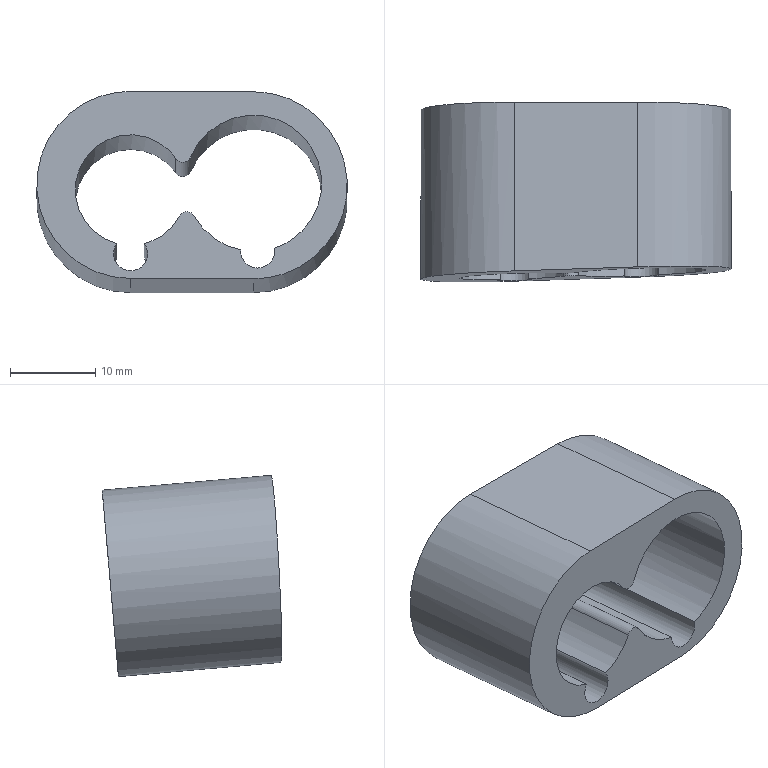Part | NX | features solid 2 | 1 solid | 14 faces | box 36.5 x 21.114 x 23.653 mm | volume 6698 mm3 | cylinder 10 | plane 4 | commonest cylinder face diameters 2 x2 4 x2 13 x2 16 x2 22 x2
STEP:
#1=CARTESIAN_POINT('',(-235.351,-38.939,-37.55));
#2=VERTEX_POINT('',#1);
#3=CARTESIAN_POINT('',(-229.897,-39.284,-41.487));
#4=VERTEX_POINT('',#3);
#5=CARTESIAN_POINT('',(-228.366,-38.599,-33.665));
#6=DIRECTION('',(0.,-0.9962,0.08716));
#7=DIRECTION('',(0.,-0.08716,-0.9962));
#8=AXIS2_PLACEMENT_3D('',#5,#6,#7);
#9=CIRCLE('',#8,8.);
#10=EDGE_CURVE('',#2,#4,#9,.T.);
#11=ORIENTED_EDGE('',*,*,#10,.F.);
#12=CARTESIAN_POINT('',(-235.351,-58.041,-35.879));
#13=VERTEX_POINT('',#12);
#14=CARTESIAN_POINT('',(-235.351,-58.346,-35.852));
#15=DIRECTION('',(0.,0.9962,-0.08716));
#16=VECTOR('',#15,1000.);
#17=LINE('',#14,#16);
#18=EDGE_CURVE('',#2,#13,#17,.F.);
#19=ORIENTED_EDGE('',*,*,#18,.T.);
#20=CARTESIAN_POINT('',(-229.897,-58.074,-39.843));
#21=VERTEX_POINT('',#20);
#22=CARTESIAN_POINT('',(-228.366,-57.608,-32.002));
#23=DIRECTION('',(-0.03252,0.9981,-0.05307));
#24=DIRECTION('',(0.6892,-0.01607,-0.7244));
#25=AXIS2_PLACEMENT_3D('',#22,#23,#24);
#26=ELLIPSE('',#25,8.009,8.);
#27=EDGE_CURVE('',#13,#21,#26,.F.);
#28=ORIENTED_EDGE('',*,*,#27,.T.);
#29=CARTESIAN_POINT('',(-229.897,-48.729,-40.661));
#30=DIRECTION('',(0.,0.9962,-0.08716));
#31=VECTOR('',#30,1000.);
#32=LINE('',#29,#31);
#33=EDGE_CURVE('',#21,#4,#32,.T.);
#34=ORIENTED_EDGE('',*,*,#33,.T.);
#35=EDGE_LOOP('',(#11,#19,#28,#34));
#36=FACE_BOUND('',#35,.T.);
#37=CARTESIAN_POINT('',(-228.366,-58.006,-31.967));
#38=DIRECTION('',(0.,0.9962,-0.08716));
#39=DIRECTION('',(-0.9997,-0.001977,-0.0226));
#40=AXIS2_PLACEMENT_3D('',#37,#38,#39);
#41=CYLINDRICAL_SURFACE('',#40,8.);
#42=ADVANCED_FACE('',(#36),#41,.F.);
#43=CARTESIAN_POINT('',(-237.502,-38.349,-30.804));
#44=VERTEX_POINT('',#43);
#45=CARTESIAN_POINT('',(-244.435,-39.222,-40.782));
#46=VERTEX_POINT('',#45);
#47=CARTESIAN_POINT('',(-242.835,-38.673,-34.506));
#48=DIRECTION('',(0.,-0.9962,0.08716));
#49=DIRECTION('',(0.,-0.08716,-0.9962));
#50=AXIS2_PLACEMENT_3D('',#47,#48,#49);
#51=CIRCLE('',#50,6.5);
#52=EDGE_CURVE('',#44,#46,#51,.T.);
#53=ORIENTED_EDGE('',*,*,#52,.F.);
#54=CARTESIAN_POINT('',(-237.502,-57.751,-29.107));
#55=VERTEX_POINT('',#54);
#56=CARTESIAN_POINT('',(-237.502,-58.196,-29.068));
#57=DIRECTION('',(0.,0.9962,-0.08716));
#58=VECTOR('',#57,1000.);
#59=LINE('',#56,#58);
#60=EDGE_CURVE('',#44,#55,#59,.F.);
#61=ORIENTED_EDGE('',*,*,#60,.T.);
#62=CARTESIAN_POINT('',(-244.435,-58.508,-39.095));
#63=VERTEX_POINT('',#62);
#64=CARTESIAN_POINT('',(-242.835,-58.122,-32.805));
#65=DIRECTION('',(-0.03252,0.9981,-0.05307));
#66=DIRECTION('',(0.6892,-0.01607,-0.7244));
#67=AXIS2_PLACEMENT_3D('',#64,#65,#66);
#68=ELLIPSE('',#67,6.507,6.5);
#69=EDGE_CURVE('',#55,#63,#68,.F.);
#70=ORIENTED_EDGE('',*,*,#69,.T.);
#71=CARTESIAN_POINT('',(-244.435,-49.107,-39.917));
#72=DIRECTION('',(0.,0.9962,-0.08716));
#73=VECTOR('',#72,1000.);
#74=LINE('',#71,#73);
#75=EDGE_CURVE('',#63,#46,#74,.T.);
#76=ORIENTED_EDGE('',*,*,#75,.T.);
#77=EDGE_LOOP('',(#53,#61,#70,#76));
#78=FACE_BOUND('',#77,.T.);
#79=CARTESIAN_POINT('',(-242.835,-58.52,-32.77));
#80=DIRECTION('',(0.,0.9962,-0.08716));
#81=DIRECTION('',(1.,0.,0.));
#82=AXIS2_PLACEMENT_3D('',#79,#80,#81);
#83=CYLINDRICAL_SURFACE('',#82,6.5);
#84=ADVANCED_FACE('',(#78),#83,.F.);
#85=CARTESIAN_POINT('',(-228.366,-39.579,-44.865));
#86=VERTEX_POINT('',#85);
#87=CARTESIAN_POINT('',(-228.366,-37.662,-22.949));
#88=VERTEX_POINT('',#87);
#89=CARTESIAN_POINT('',(-228.366,-38.62,-33.907));
#90=DIRECTION('',(0.,-0.9962,0.08716));
#91=DIRECTION('',(1.,0.,0.));
#92=AXIS2_PLACEMENT_3D('',#89,#90,#91);
#93=CIRCLE('',#92,11.);
#94=EDGE_CURVE('',#86,#88,#93,.T.);
#95=ORIENTED_EDGE('',*,*,#94,.T.);
#96=CARTESIAN_POINT('',(-228.366,-57.036,-21.254));
#97=VERTEX_POINT('',#96);
#98=CARTESIAN_POINT('',(-228.366,-57.586,-21.206));
#99=DIRECTION('',(0.,0.9962,-0.08716));
#100=VECTOR('',#99,1000.);
#101=LINE('',#98,#100);
#102=EDGE_CURVE('',#97,#88,#101,.T.);
#103=ORIENTED_EDGE('',*,*,#102,.F.);
#104=CARTESIAN_POINT('',(-228.366,-58.205,-43.235));
#105=VERTEX_POINT('',#104);
#106=CARTESIAN_POINT('',(-228.366,-57.621,-32.244));
#107=DIRECTION('',(-0.03252,0.9981,-0.05307));
#108=DIRECTION('',(0.6892,-0.01607,-0.7244));
#109=AXIS2_PLACEMENT_3D('',#106,#107,#108);
#110=ELLIPSE('',#109,11.012,11.);
#111=EDGE_CURVE('',#105,#97,#110,.F.);
#112=ORIENTED_EDGE('',*,*,#111,.F.);
#113=CARTESIAN_POINT('',(-228.366,-59.503,-43.122));
#114=DIRECTION('',(0.,0.9962,-0.08716));
#115=VECTOR('',#114,1000.);
#116=LINE('',#113,#115);
#117=EDGE_CURVE('',#105,#86,#116,.T.);
#118=ORIENTED_EDGE('',*,*,#117,.T.);
#119=EDGE_LOOP('',(#95,#103,#112,#118));
#120=FACE_BOUND('',#119,.T.);
#121=CARTESIAN_POINT('',(-228.366,-58.544,-32.164));
#122=DIRECTION('',(0.,0.9962,-0.08716));
#123=DIRECTION('',(0.,0.08716,0.9962));
#124=AXIS2_PLACEMENT_3D('',#121,#122,#123);
#125=CYLINDRICAL_SURFACE('',#124,11.);
#126=ADVANCED_FACE('',(#120),#125,.T.);
#127=CARTESIAN_POINT('',(-242.866,-37.662,-22.949));
#128=VERTEX_POINT('',#127);
#129=CARTESIAN_POINT('',(-242.866,-37.662,-22.949));
#130=DIRECTION('',(1.,0.,0.));
#131=VECTOR('',#130,1000.);
#132=LINE('',#129,#131);
#133=EDGE_CURVE('',#128,#88,#132,.T.);
#134=ORIENTED_EDGE('',*,*,#133,.F.);
#135=CARTESIAN_POINT('',(-242.866,-57.506,-21.212));
#136=VERTEX_POINT('',#135);
#137=CARTESIAN_POINT('',(-242.866,-57.586,-21.206));
#138=DIRECTION('',(0.,0.9962,-0.08716));
#139=VECTOR('',#138,1000.);
#140=LINE('',#137,#139);
#141=EDGE_CURVE('',#136,#128,#140,.T.);
#142=ORIENTED_EDGE('',*,*,#141,.F.);
#143=CARTESIAN_POINT('',(-242.869,-57.506,-21.212));
#144=DIRECTION('',(-0.9995,-0.03241,0.002836));
#145=VECTOR('',#144,1000.);
#146=LINE('',#143,#145);
#147=EDGE_CURVE('',#136,#97,#146,.F.);
#148=ORIENTED_EDGE('',*,*,#147,.T.);
#149=ORIENTED_EDGE('',*,*,#102,.T.);
#150=EDGE_LOOP('',(#134,#142,#148,#149));
#151=FACE_BOUND('',#150,.T.);
#152=CARTESIAN_POINT('',(-242.866,-57.586,-21.206));
#153=DIRECTION('',(0.,0.08716,0.9962));
#154=DIRECTION('',(1.,0.,0.));
#155=AXIS2_PLACEMENT_3D('',#152,#153,#154);
#156=PLANE('',#155);
#157=ADVANCED_FACE('',(#151),#156,.T.);
#158=CARTESIAN_POINT('',(-242.866,-39.579,-44.865));
#159=VERTEX_POINT('',#158);
#160=CARTESIAN_POINT('',(-242.866,-38.62,-33.907));
#161=DIRECTION('',(0.,-0.9962,0.08716));
#162=DIRECTION('',(1.,0.,0.));
#163=AXIS2_PLACEMENT_3D('',#160,#161,#162);
#164=CIRCLE('',#163,11.);
#165=EDGE_CURVE('',#128,#159,#164,.T.);
#166=ORIENTED_EDGE('',*,*,#165,.T.);
#167=CARTESIAN_POINT('',(-242.866,-58.675,-43.194));
#168=VERTEX_POINT('',#167);
#169=CARTESIAN_POINT('',(-242.866,-59.503,-43.122));
#170=DIRECTION('',(0.,0.9962,-0.08716));
#171=VECTOR('',#170,1000.);
#172=LINE('',#169,#171);
#173=EDGE_CURVE('',#168,#159,#172,.T.);
#174=ORIENTED_EDGE('',*,*,#173,.F.);
#175=CARTESIAN_POINT('',(-242.866,-58.091,-32.203));
#176=DIRECTION('',(-0.03252,0.9981,-0.05307));
#177=DIRECTION('',(0.6892,-0.01607,-0.7244));
#178=AXIS2_PLACEMENT_3D('',#175,#176,#177);
#179=ELLIPSE('',#178,11.012,11.);
#180=EDGE_CURVE('',#136,#168,#179,.F.);
#181=ORIENTED_EDGE('',*,*,#180,.F.);
#182=ORIENTED_EDGE('',*,*,#141,.T.);
#183=EDGE_LOOP('',(#166,#174,#181,#182));
#184=FACE_BOUND('',#183,.T.);
#185=CARTESIAN_POINT('',(-242.866,-58.544,-32.164));
#186=DIRECTION('',(0.,0.9962,-0.08716));
#187=DIRECTION('',(0.,0.08716,0.9962));
#188=AXIS2_PLACEMENT_3D('',#185,#186,#187);
#189=CYLINDRICAL_SURFACE('',#188,11.);
#190=ADVANCED_FACE('',(#184),#189,.T.);
#191=CARTESIAN_POINT('',(-228.366,-39.579,-44.865));
#192=DIRECTION('',(-1.,0.,0.));
#193=VECTOR('',#192,1000.);
#194=LINE('',#191,#193);
#195=EDGE_CURVE('',#86,#159,#194,.T.);
#196=ORIENTED_EDGE('',*,*,#195,.F.);
#197=ORIENTED_EDGE('',*,*,#117,.F.);
#198=CARTESIAN_POINT('',(-228.409,-58.206,-43.235));
#199=DIRECTION('',(0.9995,0.03241,-0.002836));
#200=VECTOR('',#199,1000.);
#201=LINE('',#198,#200);
#202=EDGE_CURVE('',#105,#168,#201,.F.);
#203=ORIENTED_EDGE('',*,*,#202,.T.);
#204=ORIENTED_EDGE('',*,*,#173,.T.);
#205=EDGE_LOOP('',(#196,#197,#203,#204));
#206=FACE_BOUND('',#205,.T.);
#207=CARTESIAN_POINT('',(-228.366,-59.503,-43.122));
#208=DIRECTION('',(0.,-0.08716,-0.9962));
#209=DIRECTION('',(-1.,0.,0.));
#210=AXIS2_PLACEMENT_3D('',#207,#208,#209);
#211=PLANE('',#210);
#212=ADVANCED_FACE('',(#206),#211,.T.);
#213=ORIENTED_EDGE('',*,*,#27,.F.);
#214=CARTESIAN_POINT('',(-237.106,-58.099,-35.889));
#215=VERTEX_POINT('',#214);
#216=CARTESIAN_POINT('',(-236.225,-58.096,-36.363));
#217=DIRECTION('',(-0.03252,0.9981,-0.05307));
#218=DIRECTION('',(0.6892,-0.01607,-0.7244));
#219=AXIS2_PLACEMENT_3D('',#216,#217,#218);
#220=ELLIPSE('',#219,1.001,1.);
#221=EDGE_CURVE('',#13,#215,#220,.F.);
#222=ORIENTED_EDGE('',*,*,#221,.T.);
#223=CARTESIAN_POINT('',(-241.235,-58.405,-39.104));
#224=VERTEX_POINT('',#223);
#225=CARTESIAN_POINT('',(-242.835,-58.122,-32.805));
#226=DIRECTION('',(-0.03252,0.9981,-0.05307));
#227=DIRECTION('',(0.6892,-0.01607,-0.7244));
#228=AXIS2_PLACEMENT_3D('',#225,#226,#227);
#229=ELLIPSE('',#228,6.507,6.5);
#230=EDGE_CURVE('',#224,#215,#229,.F.);
#231=ORIENTED_EDGE('',*,*,#230,.F.);
#232=CARTESIAN_POINT('',(-242.835,-58.52,-40.299));
#233=DIRECTION('',(-0.03252,0.9981,-0.05307));
#234=DIRECTION('',(0.6892,-0.01607,-0.7244));
#235=AXIS2_PLACEMENT_3D('',#232,#233,#234);
#236=ELLIPSE('',#235,2.002,2.);
#237=EDGE_CURVE('',#63,#224,#236,.F.);
#238=ORIENTED_EDGE('',*,*,#237,.F.);
#239=ORIENTED_EDGE('',*,*,#69,.F.);
#240=CARTESIAN_POINT('',(-235.758,-57.685,-28.923));
#241=VERTEX_POINT('',#240);
#242=CARTESIAN_POINT('',(-236.682,-57.694,-28.538));
#243=DIRECTION('',(-0.03252,0.9981,-0.05307));
#244=DIRECTION('',(-0.6892,0.01607,0.7244));
#245=AXIS2_PLACEMENT_3D('',#242,#243,#244);
#246=ELLIPSE('',#245,1.001,1.);
#247=EDGE_CURVE('',#55,#241,#246,.F.);
#248=ORIENTED_EDGE('',*,*,#247,.T.);
#249=CARTESIAN_POINT('',(-225.935,-57.934,-39.624));
#250=VERTEX_POINT('',#249);
#251=CARTESIAN_POINT('',(-228.366,-57.608,-32.002));
#252=DIRECTION('',(-0.03252,0.9981,-0.05307));
#253=DIRECTION('',(0.6892,-0.01607,-0.7244));
#254=AXIS2_PLACEMENT_3D('',#251,#252,#253);
#255=ELLIPSE('',#254,8.009,8.);
#256=EDGE_CURVE('',#250,#241,#255,.F.);
#257=ORIENTED_EDGE('',*,*,#256,.F.);
#258=CARTESIAN_POINT('',(-227.901,-58.017,-39.983));
#259=DIRECTION('',(-0.03252,0.9981,-0.05307));
#260=DIRECTION('',(0.6892,-0.01607,-0.7244));
#261=AXIS2_PLACEMENT_3D('',#258,#259,#260);
#262=ELLIPSE('',#261,2.002,2.);
#263=EDGE_CURVE('',#21,#250,#262,.F.);
#264=ORIENTED_EDGE('',*,*,#263,.F.);
#265=EDGE_LOOP('',(#213,#222,#231,#238,#239,#248,#257,#264));
#266=FACE_BOUND('',#265,.T.);
#267=ORIENTED_EDGE('',*,*,#111,.T.);
#268=ORIENTED_EDGE('',*,*,#147,.F.);
#269=ORIENTED_EDGE('',*,*,#180,.T.);
#270=ORIENTED_EDGE('',*,*,#202,.F.);
#271=EDGE_LOOP('',(#267,#268,#269,#270));
#272=FACE_BOUND('',#271,.T.);
#273=CARTESIAN_POINT('',(-422.194,-57.948,80.353));
#274=DIRECTION('',(-0.03252,0.9981,-0.05307));
#275=DIRECTION('',(0.05223,-0.05133,-0.9973));
#276=AXIS2_PLACEMENT_3D('',#273,#274,#275);
#277=PLANE('',#276);
#278=ADVANCED_FACE('',(#266,#272),#277,.F.);
#279=CARTESIAN_POINT('',(-241.235,-39.222,-40.782));
#280=VERTEX_POINT('',#279);
#281=CARTESIAN_POINT('',(-237.106,-38.94,-37.565));
#282=VERTEX_POINT('',#281);
#283=CARTESIAN_POINT('',(-242.835,-38.673,-34.506));
#284=DIRECTION('',(0.,-0.9962,0.08716));
#285=DIRECTION('',(0.,-0.08716,-0.9962));
#286=AXIS2_PLACEMENT_3D('',#283,#284,#285);
#287=CIRCLE('',#286,6.5);
#288=EDGE_CURVE('',#280,#282,#287,.T.);
#289=ORIENTED_EDGE('',*,*,#288,.T.);
#290=CARTESIAN_POINT('',(-236.225,-38.982,-38.036));
#291=DIRECTION('',(0.,-0.9962,0.08716));
#292=DIRECTION('',(0.,-0.08716,-0.9962));
#293=AXIS2_PLACEMENT_3D('',#290,#291,#292);
#294=CIRCLE('',#293,1.);
#295=EDGE_CURVE('',#282,#2,#294,.F.);
#296=ORIENTED_EDGE('',*,*,#295,.T.);
#297=ORIENTED_EDGE('',*,*,#10,.T.);
#298=CARTESIAN_POINT('',(-225.935,-39.263,-41.257));
#299=VERTEX_POINT('',#298);
#300=CARTESIAN_POINT('',(-227.901,-39.295,-41.621));
#301=DIRECTION('',(0.,-0.9962,0.08716));
#302=DIRECTION('',(0.,-0.08716,-0.9962));
#303=AXIS2_PLACEMENT_3D('',#300,#301,#302);
#304=CIRCLE('',#303,2.);
#305=EDGE_CURVE('',#4,#299,#304,.T.);
#306=ORIENTED_EDGE('',*,*,#305,.T.);
#307=CARTESIAN_POINT('',(-235.758,-38.332,-30.616));
#308=VERTEX_POINT('',#307);
#309=CARTESIAN_POINT('',(-228.366,-38.599,-33.665));
#310=DIRECTION('',(0.,-0.9962,0.08716));
#311=DIRECTION('',(0.,-0.08716,-0.9962));
#312=AXIS2_PLACEMENT_3D('',#309,#310,#311);
#313=CIRCLE('',#312,8.);
#314=EDGE_CURVE('',#299,#308,#313,.T.);
#315=ORIENTED_EDGE('',*,*,#314,.T.);
#316=CARTESIAN_POINT('',(-236.682,-38.299,-30.235));
#317=DIRECTION('',(0.,-0.9962,0.08716));
#318=DIRECTION('',(0.,-0.08716,-0.9962));
#319=AXIS2_PLACEMENT_3D('',#316,#317,#318);
#320=CIRCLE('',#319,1.);
#321=EDGE_CURVE('',#308,#44,#320,.F.);
#322=ORIENTED_EDGE('',*,*,#321,.T.);
#323=ORIENTED_EDGE('',*,*,#52,.T.);
#324=CARTESIAN_POINT('',(-242.835,-39.326,-41.978));
#325=DIRECTION('',(0.,-0.9962,0.08716));
#326=DIRECTION('',(0.,-0.08716,-0.9962));
#327=AXIS2_PLACEMENT_3D('',#324,#325,#326);
#328=CIRCLE('',#327,2.);
#329=EDGE_CURVE('',#46,#280,#328,.T.);
#330=ORIENTED_EDGE('',*,*,#329,.T.);
#331=EDGE_LOOP('',(#289,#296,#297,#306,#315,#322,#323,#330));
#332=FACE_BOUND('',#331,.T.);
#333=ORIENTED_EDGE('',*,*,#94,.F.);
#334=ORIENTED_EDGE('',*,*,#195,.T.);
#335=ORIENTED_EDGE('',*,*,#165,.F.);
#336=ORIENTED_EDGE('',*,*,#133,.T.);
#337=EDGE_LOOP('',(#333,#334,#335,#336));
#338=FACE_BOUND('',#337,.T.);
#339=CARTESIAN_POINT('',(-228.366,-38.62,-33.907));
#340=DIRECTION('',(0.,-0.9962,0.08716));
#341=DIRECTION('',(0.,-0.08716,-0.9962));
#342=AXIS2_PLACEMENT_3D('',#339,#340,#341);
#343=PLANE('',#342);
#344=ADVANCED_FACE('',(#332,#338),#343,.F.);
#345=ORIENTED_EDGE('',*,*,#230,.T.);
#346=CARTESIAN_POINT('',(-237.106,-58.788,-35.829));
#347=DIRECTION('',(0.,0.9962,-0.08716));
#348=VECTOR('',#347,1000.);
#349=LINE('',#346,#348);
#350=EDGE_CURVE('',#215,#282,#349,.T.);
#351=ORIENTED_EDGE('',*,*,#350,.T.);
#352=ORIENTED_EDGE('',*,*,#288,.F.);
#353=CARTESIAN_POINT('',(-241.235,-49.107,-39.917));
#354=DIRECTION('',(0.,0.9962,-0.08716));
#355=VECTOR('',#354,1000.);
#356=LINE('',#353,#355);
#357=EDGE_CURVE('',#280,#224,#356,.F.);
#358=ORIENTED_EDGE('',*,*,#357,.T.);
#359=EDGE_LOOP('',(#345,#351,#352,#358));
#360=FACE_BOUND('',#359,.T.);
#361=CARTESIAN_POINT('',(-242.835,-58.52,-32.77));
#362=DIRECTION('',(0.,0.9962,-0.08716));
#363=DIRECTION('',(1.,0.,0.));
#364=AXIS2_PLACEMENT_3D('',#361,#362,#363);
#365=CYLINDRICAL_SURFACE('',#364,6.5);
#366=ADVANCED_FACE('',(#360),#365,.F.);
#367=ORIENTED_EDGE('',*,*,#256,.T.);
#368=CARTESIAN_POINT('',(-235.758,-57.739,-28.918));
#369=DIRECTION('',(0.,0.9962,-0.08716));
#370=VECTOR('',#369,1000.);
#371=LINE('',#368,#370);
#372=EDGE_CURVE('',#241,#308,#371,.T.);
#373=ORIENTED_EDGE('',*,*,#372,.T.);
#374=ORIENTED_EDGE('',*,*,#314,.F.);
#375=CARTESIAN_POINT('',(-225.935,-48.708,-40.431));
#376=DIRECTION('',(0.,0.9962,-0.08716));
#377=VECTOR('',#376,1000.);
#378=LINE('',#375,#377);
#379=EDGE_CURVE('',#299,#250,#378,.F.);
#380=ORIENTED_EDGE('',*,*,#379,.T.);
#381=EDGE_LOOP('',(#367,#373,#374,#380));
#382=FACE_BOUND('',#381,.T.);
#383=CARTESIAN_POINT('',(-228.366,-58.006,-31.967));
#384=DIRECTION('',(0.,0.9962,-0.08716));
#385=DIRECTION('',(-0.9997,-0.001977,-0.0226));
#386=AXIS2_PLACEMENT_3D('',#383,#384,#385);
#387=CYLINDRICAL_SURFACE('',#386,8.);
#388=ADVANCED_FACE('',(#382),#387,.F.);
#389=ORIENTED_EDGE('',*,*,#237,.T.);
#390=ORIENTED_EDGE('',*,*,#357,.F.);
#391=ORIENTED_EDGE('',*,*,#329,.F.);
#392=ORIENTED_EDGE('',*,*,#75,.F.);
#393=EDGE_LOOP('',(#389,#390,#391,#392));
#394=FACE_BOUND('',#393,.T.);
#395=CARTESIAN_POINT('',(-242.835,-59.174,-40.241));
#396=DIRECTION('',(0.,0.9962,-0.08716));
#397=DIRECTION('',(1.,0.,0.));
#398=AXIS2_PLACEMENT_3D('',#395,#396,#397);
#399=CYLINDRICAL_SURFACE('',#398,2.);
#400=ADVANCED_FACE('',(#394),#399,.F.);
#401=ORIENTED_EDGE('',*,*,#263,.T.);
#402=ORIENTED_EDGE('',*,*,#379,.F.);
#403=ORIENTED_EDGE('',*,*,#305,.F.);
#404=ORIENTED_EDGE('',*,*,#33,.F.);
#405=EDGE_LOOP('',(#401,#402,#403,#404));
#406=FACE_BOUND('',#405,.T.);
#407=CARTESIAN_POINT('',(-227.901,-58.702,-39.923));
#408=DIRECTION('',(0.,0.9962,-0.08716));
#409=DIRECTION('',(-0.9997,-0.001977,-0.0226));
#410=AXIS2_PLACEMENT_3D('',#407,#408,#409);
#411=CYLINDRICAL_SURFACE('',#410,2.);
#412=ADVANCED_FACE('',(#406),#411,.F.);
#413=ORIENTED_EDGE('',*,*,#321,.F.);
#414=ORIENTED_EDGE('',*,*,#372,.F.);
#415=ORIENTED_EDGE('',*,*,#247,.F.);
#416=ORIENTED_EDGE('',*,*,#60,.F.);
#417=EDGE_LOOP('',(#413,#414,#415,#416));
#418=FACE_BOUND('',#417,.T.);
#419=CARTESIAN_POINT('',(-236.682,-57.706,-28.537));
#420=DIRECTION('',(0.,-0.9962,0.08716));
#421=DIRECTION('',(0.,-0.08716,-0.9962));
#422=AXIS2_PLACEMENT_3D('',#419,#420,#421);
#423=CYLINDRICAL_SURFACE('',#422,1.);
#424=ADVANCED_FACE('',(#418),#423,.T.);
#425=ORIENTED_EDGE('',*,*,#221,.F.);
#426=ORIENTED_EDGE('',*,*,#18,.F.);
#427=ORIENTED_EDGE('',*,*,#295,.F.);
#428=ORIENTED_EDGE('',*,*,#350,.F.);
#429=EDGE_LOOP('',(#425,#426,#427,#428));
#430=FACE_BOUND('',#429,.T.);
#431=CARTESIAN_POINT('',(-236.225,-58.388,-36.338));
#432=DIRECTION('',(0.,0.9962,-0.08716));
#433=DIRECTION('',(0.,0.08716,0.9962));
#434=AXIS2_PLACEMENT_3D('',#431,#432,#433);
#435=CYLINDRICAL_SURFACE('',#434,1.);
#436=ADVANCED_FACE('',(#430),#435,.T.);
#437=CLOSED_SHELL('',(#42,#84,#126,#157,#190,#212,#278,#344,#366,#388,#400,#412,#424,#436));
#438=MANIFOLD_SOLID_BREP('',#437);
#439=(LENGTH_UNIT()NAMED_UNIT(*)SI_UNIT(.MILLI.,.METRE.));
#440=UNCERTAINTY_MEASURE_WITH_UNIT(LENGTH_MEASURE(0.00001),#439,'','');
#441=(NAMED_UNIT(*)PLANE_ANGLE_UNIT()SI_UNIT($,.RADIAN.));
#442=(NAMED_UNIT(*)SI_UNIT($,.STERADIAN.)SOLID_ANGLE_UNIT());
#443=(GEOMETRIC_REPRESENTATION_CONTEXT(3)GLOBAL_UNCERTAINTY_ASSIGNED_CONTEXT((#440))GLOBAL_UNIT_ASSIGNED_CONTEXT((#439,#441,#442))REPRESENTATION_CONTEXT('',''));
#444=ADVANCED_BREP_SHAPE_REPRESENTATION('',(#438),#443);